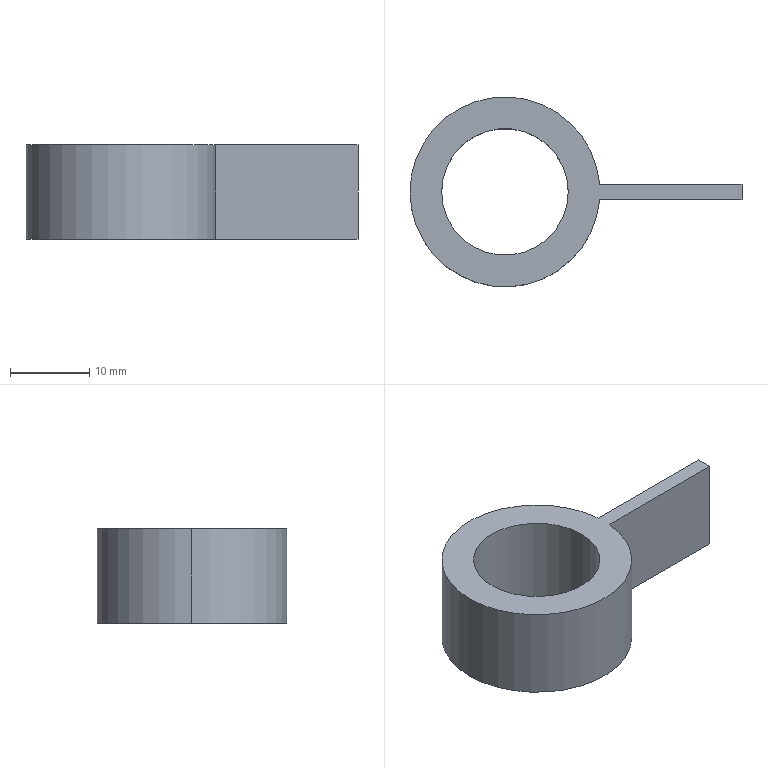Part | SolidWorks | features Extrusion 1, ICE 1 | 1 solid | 9 faces | box 41.958 x 24 x 12 mm | volume 3447 mm3 | plane 5 | cylinder 4 | commonest cylinder face diameters 16 x2 24 x2
STEP:
#1=CARTESIAN_POINT('',(-8.,0.,6.));
#2=VERTEX_POINT('',#1);
#3=CARTESIAN_POINT('',(8.,0.,6.));
#4=VERTEX_POINT('',#3);
#5=CARTESIAN_POINT('',(0.,0.,6.));
#6=DIRECTION('',(0.,0.,1.));
#7=DIRECTION('',(1.,0.,0.));
#8=AXIS2_PLACEMENT_3D('',#5,#6,#7);
#9=CIRCLE('',#8,8.);
#10=EDGE_CURVE('',#2,#4,#9,.T.);
#11=ORIENTED_EDGE('',*,*,#10,.T.);
#12=CARTESIAN_POINT('',(8.,0.,-6.));
#13=VERTEX_POINT('',#12);
#14=CARTESIAN_POINT('',(8.,0.,6.));
#15=DIRECTION('',(0.,0.,-1.));
#16=VECTOR('',#15,1000.);
#17=LINE('',#14,#16);
#18=EDGE_CURVE('',#4,#13,#17,.T.);
#19=ORIENTED_EDGE('',*,*,#18,.T.);
#20=CARTESIAN_POINT('',(-8.,0.,-6.));
#21=VERTEX_POINT('',#20);
#22=CARTESIAN_POINT('',(0.,0.,-6.));
#23=DIRECTION('',(0.,0.,1.));
#24=DIRECTION('',(1.,0.,0.));
#25=AXIS2_PLACEMENT_3D('',#22,#23,#24);
#26=CIRCLE('',#25,8.);
#27=EDGE_CURVE('',#21,#13,#26,.T.);
#28=ORIENTED_EDGE('',*,*,#27,.F.);
#29=CARTESIAN_POINT('',(-8.,0.,6.));
#30=DIRECTION('',(0.,0.,-1.));
#31=VECTOR('',#30,1000.);
#32=LINE('',#29,#31);
#33=EDGE_CURVE('',#2,#21,#32,.T.);
#34=ORIENTED_EDGE('',*,*,#33,.F.);
#35=EDGE_LOOP('',(#11,#19,#28,#34));
#36=FACE_OUTER_BOUND('',#35,.T.);
#37=CARTESIAN_POINT('',(0.,0.,6.));
#38=DIRECTION('',(0.,0.,-1.));
#39=DIRECTION('',(-1.,0.,0.));
#40=AXIS2_PLACEMENT_3D('',#37,#38,#39);
#41=CYLINDRICAL_SURFACE('',#40,8.);
#42=ADVANCED_FACE('',(#36),#41,.F.);
#43=CARTESIAN_POINT('',(-12.,0.,6.));
#44=VERTEX_POINT('',#43);
#45=CARTESIAN_POINT('',(11.958,-1.,6.));
#46=VERTEX_POINT('',#45);
#47=CARTESIAN_POINT('',(0.,0.,6.));
#48=DIRECTION('',(0.,0.,1.));
#49=DIRECTION('',(1.,0.,0.));
#50=AXIS2_PLACEMENT_3D('',#47,#48,#49);
#51=CIRCLE('',#50,12.);
#52=EDGE_CURVE('',#44,#46,#51,.T.);
#53=ORIENTED_EDGE('',*,*,#52,.F.);
#54=CARTESIAN_POINT('',(-12.,0.,-6.));
#55=VERTEX_POINT('',#54);
#56=CARTESIAN_POINT('',(-12.,0.,6.));
#57=DIRECTION('',(0.,0.,-1.));
#58=VECTOR('',#57,1000.);
#59=LINE('',#56,#58);
#60=EDGE_CURVE('',#44,#55,#59,.T.);
#61=ORIENTED_EDGE('',*,*,#60,.T.);
#62=CARTESIAN_POINT('',(11.958,-1.,-6.));
#63=VERTEX_POINT('',#62);
#64=CARTESIAN_POINT('',(0.,0.,-6.));
#65=DIRECTION('',(0.,0.,1.));
#66=DIRECTION('',(1.,0.,0.));
#67=AXIS2_PLACEMENT_3D('',#64,#65,#66);
#68=CIRCLE('',#67,12.);
#69=EDGE_CURVE('',#55,#63,#68,.T.);
#70=ORIENTED_EDGE('',*,*,#69,.T.);
#71=CARTESIAN_POINT('',(11.958,-1.,-24.111));
#72=DIRECTION('',(0.,0.,1.));
#73=VECTOR('',#72,1000.);
#74=LINE('',#71,#73);
#75=EDGE_CURVE('',#63,#46,#74,.T.);
#76=ORIENTED_EDGE('',*,*,#75,.T.);
#77=EDGE_LOOP('',(#53,#61,#70,#76));
#78=FACE_OUTER_BOUND('',#77,.T.);
#79=CARTESIAN_POINT('',(0.,0.,6.));
#80=DIRECTION('',(0.,0.,-1.));
#81=DIRECTION('',(-1.,0.,0.));
#82=AXIS2_PLACEMENT_3D('',#79,#80,#81);
#83=CYLINDRICAL_SURFACE('',#82,12.);
#84=ADVANCED_FACE('',(#78),#83,.T.);
#85=CARTESIAN_POINT('',(11.958,1.,6.));
#86=VERTEX_POINT('',#85);
#87=CARTESIAN_POINT('',(0.,0.,6.));
#88=DIRECTION('',(0.,0.,1.));
#89=DIRECTION('',(1.,0.,0.));
#90=AXIS2_PLACEMENT_3D('',#87,#88,#89);
#91=CIRCLE('',#90,12.);
#92=EDGE_CURVE('',#86,#44,#91,.T.);
#93=ORIENTED_EDGE('',*,*,#92,.T.);
#94=ORIENTED_EDGE('',*,*,#52,.T.);
#95=CARTESIAN_POINT('',(29.958,-1.,6.));
#96=VERTEX_POINT('',#95);
#97=CARTESIAN_POINT('',(29.958,-1.,6.));
#98=DIRECTION('',(1.,0.,0.));
#99=VECTOR('',#98,1000.);
#100=LINE('',#97,#99);
#101=EDGE_CURVE('',#46,#96,#100,.T.);
#102=ORIENTED_EDGE('',*,*,#101,.T.);
#103=CARTESIAN_POINT('',(29.958,1.,6.));
#104=VERTEX_POINT('',#103);
#105=CARTESIAN_POINT('',(29.958,1.,6.));
#106=DIRECTION('',(0.,1.,0.));
#107=VECTOR('',#106,1000.);
#108=LINE('',#105,#107);
#109=EDGE_CURVE('',#96,#104,#108,.T.);
#110=ORIENTED_EDGE('',*,*,#109,.T.);
#111=CARTESIAN_POINT('',(11.958,1.,6.));
#112=DIRECTION('',(-1.,0.,0.));
#113=VECTOR('',#112,1000.);
#114=LINE('',#111,#113);
#115=EDGE_CURVE('',#104,#86,#114,.T.);
#116=ORIENTED_EDGE('',*,*,#115,.T.);
#117=EDGE_LOOP('',(#93,#94,#102,#110,#116));
#118=FACE_OUTER_BOUND('',#117,.T.);
#119=ORIENTED_EDGE('',*,*,#10,.F.);
#120=CARTESIAN_POINT('',(0.,0.,6.));
#121=DIRECTION('',(0.,0.,1.));
#122=DIRECTION('',(1.,0.,0.));
#123=AXIS2_PLACEMENT_3D('',#120,#121,#122);
#124=CIRCLE('',#123,8.);
#125=EDGE_CURVE('',#4,#2,#124,.T.);
#126=ORIENTED_EDGE('',*,*,#125,.F.);
#127=EDGE_LOOP('',(#119,#126));
#128=FACE_BOUND('',#127,.T.);
#129=CARTESIAN_POINT('',(0.,0.,6.));
#130=DIRECTION('',(0.,0.,1.));
#131=DIRECTION('',(1.,0.,0.));
#132=AXIS2_PLACEMENT_3D('',#129,#130,#131);
#133=PLANE('',#132);
#134=ADVANCED_FACE('',(#118,#128),#133,.T.);
#135=CARTESIAN_POINT('',(11.958,1.,-6.));
#136=VERTEX_POINT('',#135);
#137=CARTESIAN_POINT('',(0.,0.,-6.));
#138=DIRECTION('',(0.,0.,1.));
#139=DIRECTION('',(1.,0.,0.));
#140=AXIS2_PLACEMENT_3D('',#137,#138,#139);
#141=CIRCLE('',#140,12.);
#142=EDGE_CURVE('',#136,#55,#141,.T.);
#143=ORIENTED_EDGE('',*,*,#142,.F.);
#144=CARTESIAN_POINT('',(29.958,1.,-6.));
#145=VERTEX_POINT('',#144);
#146=CARTESIAN_POINT('',(11.958,1.,-6.));
#147=DIRECTION('',(1.,0.,0.));
#148=VECTOR('',#147,1000.);
#149=LINE('',#146,#148);
#150=EDGE_CURVE('',#136,#145,#149,.T.);
#151=ORIENTED_EDGE('',*,*,#150,.T.);
#152=CARTESIAN_POINT('',(29.958,-1.,-6.));
#153=VERTEX_POINT('',#152);
#154=CARTESIAN_POINT('',(29.958,1.,-6.));
#155=DIRECTION('',(0.,-1.,0.));
#156=VECTOR('',#155,1000.);
#157=LINE('',#154,#156);
#158=EDGE_CURVE('',#145,#153,#157,.T.);
#159=ORIENTED_EDGE('',*,*,#158,.T.);
#160=CARTESIAN_POINT('',(29.958,-1.,-6.));
#161=DIRECTION('',(-1.,0.,0.));
#162=VECTOR('',#161,1000.);
#163=LINE('',#160,#162);
#164=EDGE_CURVE('',#153,#63,#163,.T.);
#165=ORIENTED_EDGE('',*,*,#164,.T.);
#166=ORIENTED_EDGE('',*,*,#69,.F.);
#167=EDGE_LOOP('',(#143,#151,#159,#165,#166));
#168=FACE_OUTER_BOUND('',#167,.T.);
#169=ORIENTED_EDGE('',*,*,#27,.T.);
#170=CARTESIAN_POINT('',(0.,0.,-6.));
#171=DIRECTION('',(0.,0.,1.));
#172=DIRECTION('',(1.,0.,0.));
#173=AXIS2_PLACEMENT_3D('',#170,#171,#172);
#174=CIRCLE('',#173,8.);
#175=EDGE_CURVE('',#13,#21,#174,.T.);
#176=ORIENTED_EDGE('',*,*,#175,.T.);
#177=EDGE_LOOP('',(#169,#176));
#178=FACE_BOUND('',#177,.T.);
#179=CARTESIAN_POINT('',(0.,0.,-6.));
#180=DIRECTION('',(0.,0.,1.));
#181=DIRECTION('',(1.,0.,0.));
#182=AXIS2_PLACEMENT_3D('',#179,#180,#181);
#183=PLANE('',#182);
#184=ADVANCED_FACE('',(#168,#178),#183,.F.);
#185=ORIENTED_EDGE('',*,*,#60,.F.);
#186=ORIENTED_EDGE('',*,*,#92,.F.);
#187=CARTESIAN_POINT('',(11.958,1.,-24.111));
#188=DIRECTION('',(0.,0.,1.));
#189=VECTOR('',#188,1000.);
#190=LINE('',#187,#189);
#191=EDGE_CURVE('',#136,#86,#190,.T.);
#192=ORIENTED_EDGE('',*,*,#191,.F.);
#193=ORIENTED_EDGE('',*,*,#142,.T.);
#194=EDGE_LOOP('',(#185,#186,#192,#193));
#195=FACE_OUTER_BOUND('',#194,.T.);
#196=CARTESIAN_POINT('',(0.,0.,6.));
#197=DIRECTION('',(0.,0.,-1.));
#198=DIRECTION('',(-1.,0.,0.));
#199=AXIS2_PLACEMENT_3D('',#196,#197,#198);
#200=CYLINDRICAL_SURFACE('',#199,12.);
#201=ADVANCED_FACE('',(#195),#200,.T.);
#202=ORIENTED_EDGE('',*,*,#18,.F.);
#203=ORIENTED_EDGE('',*,*,#125,.T.);
#204=ORIENTED_EDGE('',*,*,#33,.T.);
#205=ORIENTED_EDGE('',*,*,#175,.F.);
#206=EDGE_LOOP('',(#202,#203,#204,#205));
#207=FACE_OUTER_BOUND('',#206,.T.);
#208=CARTESIAN_POINT('',(0.,0.,6.));
#209=DIRECTION('',(0.,0.,-1.));
#210=DIRECTION('',(-1.,0.,0.));
#211=AXIS2_PLACEMENT_3D('',#208,#209,#210);
#212=CYLINDRICAL_SURFACE('',#211,8.);
#213=ADVANCED_FACE('',(#207),#212,.F.);
#214=ORIENTED_EDGE('',*,*,#150,.F.);
#215=ORIENTED_EDGE('',*,*,#191,.T.);
#216=ORIENTED_EDGE('',*,*,#115,.F.);
#217=CARTESIAN_POINT('',(29.958,1.,-24.111));
#218=DIRECTION('',(0.,0.,1.));
#219=VECTOR('',#218,1000.);
#220=LINE('',#217,#219);
#221=EDGE_CURVE('',#145,#104,#220,.T.);
#222=ORIENTED_EDGE('',*,*,#221,.F.);
#223=EDGE_LOOP('',(#214,#215,#216,#222));
#224=FACE_OUTER_BOUND('',#223,.T.);
#225=CARTESIAN_POINT('',(11.958,1.,-24.111));
#226=DIRECTION('',(0.,1.,0.));
#227=DIRECTION('',(0.,0.,1.));
#228=AXIS2_PLACEMENT_3D('',#225,#226,#227);
#229=PLANE('',#228);
#230=ADVANCED_FACE('',(#224),#229,.T.);
#231=ORIENTED_EDGE('',*,*,#158,.F.);
#232=ORIENTED_EDGE('',*,*,#221,.T.);
#233=ORIENTED_EDGE('',*,*,#109,.F.);
#234=CARTESIAN_POINT('',(29.958,-1.,-24.111));
#235=DIRECTION('',(0.,0.,1.));
#236=VECTOR('',#235,1000.);
#237=LINE('',#234,#236);
#238=EDGE_CURVE('',#153,#96,#237,.T.);
#239=ORIENTED_EDGE('',*,*,#238,.F.);
#240=EDGE_LOOP('',(#231,#232,#233,#239));
#241=FACE_OUTER_BOUND('',#240,.T.);
#242=CARTESIAN_POINT('',(29.958,1.,-24.111));
#243=DIRECTION('',(1.,0.,0.));
#244=DIRECTION('',(0.,0.,-1.));
#245=AXIS2_PLACEMENT_3D('',#242,#243,#244);
#246=PLANE('',#245);
#247=ADVANCED_FACE('',(#241),#246,.T.);
#248=ORIENTED_EDGE('',*,*,#164,.F.);
#249=ORIENTED_EDGE('',*,*,#238,.T.);
#250=ORIENTED_EDGE('',*,*,#101,.F.);
#251=ORIENTED_EDGE('',*,*,#75,.F.);
#252=EDGE_LOOP('',(#248,#249,#250,#251));
#253=FACE_OUTER_BOUND('',#252,.T.);
#254=CARTESIAN_POINT('',(29.958,-1.,-24.111));
#255=DIRECTION('',(0.,-1.,0.));
#256=DIRECTION('',(0.,0.,-1.));
#257=AXIS2_PLACEMENT_3D('',#254,#255,#256);
#258=PLANE('',#257);
#259=ADVANCED_FACE('',(#253),#258,.T.);
#260=CLOSED_SHELL('',(#42,#84,#134,#184,#201,#213,#230,#247,#259));
#261=MANIFOLD_SOLID_BREP('',#260);
#262=CARTESIAN_POINT('',(0.,0.,0.));
#263=DIRECTION('',(0.,0.,1.));
#264=DIRECTION('',(1.,0.,0.));
#265=AXIS2_PLACEMENT_3D('',#262,#263,#264);
#266=(LENGTH_UNIT()NAMED_UNIT(*)SI_UNIT(.MILLI.,.METRE.));
#267=UNCERTAINTY_MEASURE_WITH_UNIT(LENGTH_MEASURE(0.00001),#266,'','');
#268=(NAMED_UNIT(*)PLANE_ANGLE_UNIT()SI_UNIT($,.RADIAN.));
#269=(NAMED_UNIT(*)SI_UNIT($,.STERADIAN.)SOLID_ANGLE_UNIT());
#270=(GEOMETRIC_REPRESENTATION_CONTEXT(3)GLOBAL_UNCERTAINTY_ASSIGNED_CONTEXT((#267))GLOBAL_UNIT_ASSIGNED_CONTEXT((#266,#268,#269))REPRESENTATION_CONTEXT('',''));
#271=ADVANCED_BREP_SHAPE_REPRESENTATION('',(#261,#265),#270);